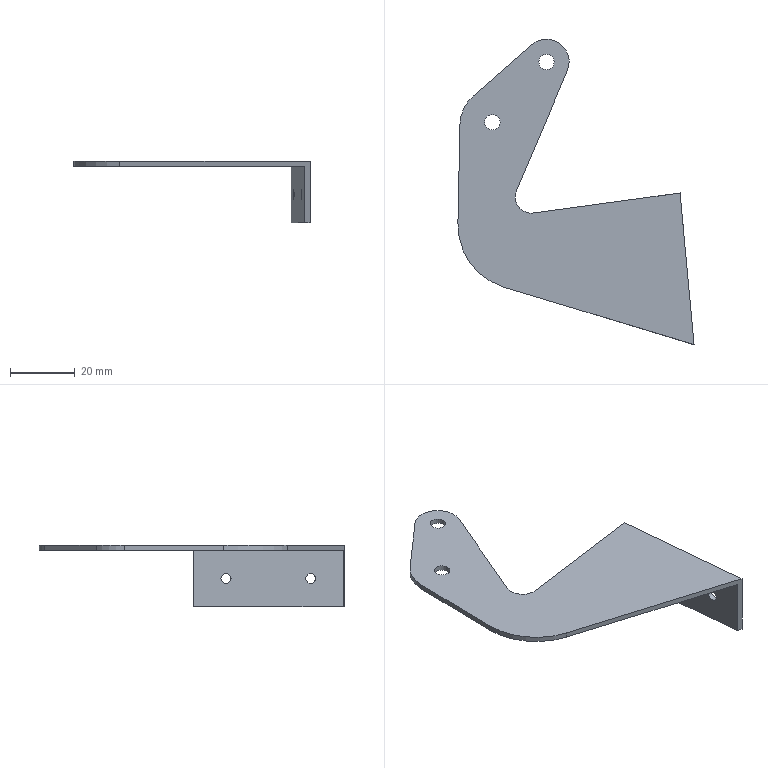Part | NX | features door hinge 2(right) 2 | 1 solid | 18 faces | box 72.896 x 94.255 x 19 mm | volume 6406 mm3 | plane 10 | cylinder 8 | commonest cylinder face diameters 3.175 x2 4.762 x1 4.763 x1 10 x1 14 x1 24 x1
STEP:
#1=CARTESIAN_POINT('',(6.443,-2.735,-1.575));
#2=VERTEX_POINT('',#1);
#3=CARTESIAN_POINT('',(6.443,-2.735,0.));
#4=VERTEX_POINT('',#3);
#5=CARTESIAN_POINT('',(6.443,-2.735,-19.));
#6=DIRECTION('',(0.,0.,1.));
#7=VECTOR('',#6,1000.);
#8=LINE('',#5,#7);
#9=EDGE_CURVE('',#2,#4,#8,.T.);
#10=ORIENTED_EDGE('',*,*,#9,.F.);
#11=CARTESIAN_POINT('',(-4.613,5.265,-1.575));
#12=VERTEX_POINT('',#11);
#13=CARTESIAN_POINT('',(0.,0.,-1.575));
#14=DIRECTION('',(0.,0.,1.));
#15=DIRECTION('',(1.,0.,0.));
#16=AXIS2_PLACEMENT_3D('',#13,#14,#15);
#17=CIRCLE('',#16,7.);
#18=EDGE_CURVE('',#2,#12,#17,.T.);
#19=ORIENTED_EDGE('',*,*,#18,.T.);
#20=CARTESIAN_POINT('',(-4.613,5.265,0.));
#21=VERTEX_POINT('',#20);
#22=CARTESIAN_POINT('',(-4.613,5.265,-19.));
#23=DIRECTION('',(0.,0.,1.));
#24=VECTOR('',#23,1000.);
#25=LINE('',#22,#24);
#26=EDGE_CURVE('',#12,#21,#25,.T.);
#27=ORIENTED_EDGE('',*,*,#26,.T.);
#28=CARTESIAN_POINT('',(0.,0.,0.));
#29=DIRECTION('',(0.,0.,1.));
#30=DIRECTION('',(1.,0.,0.));
#31=AXIS2_PLACEMENT_3D('',#28,#29,#30);
#32=CIRCLE('',#31,7.);
#33=EDGE_CURVE('',#4,#21,#32,.T.);
#34=ORIENTED_EDGE('',*,*,#33,.F.);
#35=EDGE_LOOP('',(#10,#19,#27,#34));
#36=FACE_BOUND('',#35,.T.);
#37=CARTESIAN_POINT('',(0.,0.,-19.));
#38=DIRECTION('',(0.,0.,1.));
#39=DIRECTION('',(1.,0.,0.));
#40=AXIS2_PLACEMENT_3D('',#37,#38,#39);
#41=CYLINDRICAL_SURFACE('',#40,7.);
#42=ADVANCED_FACE('',(#36),#41,.T.);
#43=CARTESIAN_POINT('',(-9.254,-39.713,-1.575));
#44=VERTEX_POINT('',#43);
#45=CARTESIAN_POINT('',(-9.254,-39.713,0.));
#46=VERTEX_POINT('',#45);
#47=CARTESIAN_POINT('',(-9.254,-39.713,-19.));
#48=DIRECTION('',(0.,0.,1.));
#49=VECTOR('',#48,1000.);
#50=LINE('',#47,#49);
#51=EDGE_CURVE('',#44,#46,#50,.T.);
#52=ORIENTED_EDGE('',*,*,#51,.F.);
#53=CARTESIAN_POINT('',(6.443,-2.735,-1.575));
#54=DIRECTION('',(0.3908,0.9205,0.));
#55=VECTOR('',#54,1000.);
#56=LINE('',#53,#55);
#57=EDGE_CURVE('',#44,#2,#56,.T.);
#58=ORIENTED_EDGE('',*,*,#57,.T.);
#59=ORIENTED_EDGE('',*,*,#9,.T.);
#60=CARTESIAN_POINT('',(6.443,-2.735,0.));
#61=DIRECTION('',(0.3908,0.9205,0.));
#62=VECTOR('',#61,1000.);
#63=LINE('',#60,#62);
#64=EDGE_CURVE('',#46,#4,#63,.T.);
#65=ORIENTED_EDGE('',*,*,#64,.F.);
#66=EDGE_LOOP('',(#52,#58,#59,#65));
#67=FACE_BOUND('',#66,.T.);
#68=CARTESIAN_POINT('',(6.443,-2.735,-19.));
#69=DIRECTION('',(0.9205,-0.3908,0.));
#70=DIRECTION('',(0.3908,0.9205,0.));
#71=AXIS2_PLACEMENT_3D('',#68,#69,#70);
#72=PLANE('',#71);
#73=ADVANCED_FACE('',(#67),#72,.T.);
#74=CARTESIAN_POINT('',(-3.976,-46.621,-1.575));
#75=VERTEX_POINT('',#74);
#76=CARTESIAN_POINT('',(-3.976,-46.621,0.));
#77=VERTEX_POINT('',#76);
#78=CARTESIAN_POINT('',(-3.976,-46.621,-19.));
#79=DIRECTION('',(0.,0.,1.));
#80=VECTOR('',#79,1000.);
#81=LINE('',#78,#80);
#82=EDGE_CURVE('',#75,#77,#81,.T.);
#83=ORIENTED_EDGE('',*,*,#82,.F.);
#84=CARTESIAN_POINT('',(-4.652,-41.667,-1.575));
#85=DIRECTION('',(0.,0.,1.));
#86=DIRECTION('',(1.,0.,0.));
#87=AXIS2_PLACEMENT_3D('',#84,#85,#86);
#88=CIRCLE('',#87,5.);
#89=EDGE_CURVE('',#75,#44,#88,.F.);
#90=ORIENTED_EDGE('',*,*,#89,.T.);
#91=ORIENTED_EDGE('',*,*,#51,.T.);
#92=CARTESIAN_POINT('',(-4.652,-41.667,0.));
#93=DIRECTION('',(0.,0.,-1.));
#94=DIRECTION('',(1.,0.,0.));
#95=AXIS2_PLACEMENT_3D('',#92,#93,#94);
#96=CIRCLE('',#95,5.);
#97=EDGE_CURVE('',#77,#46,#96,.T.);
#98=ORIENTED_EDGE('',*,*,#97,.F.);
#99=EDGE_LOOP('',(#83,#90,#91,#98));
#100=FACE_BOUND('',#99,.T.);
#101=CARTESIAN_POINT('',(-4.652,-41.667,-19.));
#102=DIRECTION('',(0.,0.,1.));
#103=DIRECTION('',(1.,0.,0.));
#104=AXIS2_PLACEMENT_3D('',#101,#102,#103);
#105=CYLINDRICAL_SURFACE('',#104,5.);
#106=ADVANCED_FACE('',(#100),#105,.F.);
#107=CARTESIAN_POINT('',(39.663,-40.665,-19.));
#108=VERTEX_POINT('',#107);
#109=CARTESIAN_POINT('',(39.663,-40.665,-1.575));
#110=VERTEX_POINT('',#109);
#111=CARTESIAN_POINT('',(39.663,-40.665,-1.575));
#112=DIRECTION('',(0.,0.,1.));
#113=VECTOR('',#112,1000.);
#114=LINE('',#111,#113);
#115=EDGE_CURVE('',#108,#110,#114,.T.);
#116=ORIENTED_EDGE('',*,*,#115,.T.);
#117=CARTESIAN_POINT('',(6.175,-45.236,-1.575));
#118=DIRECTION('',(-0.9908,-0.1352,0.));
#119=VECTOR('',#118,1000.);
#120=LINE('',#117,#119);
#121=EDGE_CURVE('',#110,#75,#120,.T.);
#122=ORIENTED_EDGE('',*,*,#121,.T.);
#123=ORIENTED_EDGE('',*,*,#82,.T.);
#124=CARTESIAN_POINT('',(41.225,-40.452,0.));
#125=VERTEX_POINT('',#124);
#126=CARTESIAN_POINT('',(-3.976,-46.621,0.));
#127=DIRECTION('',(-0.9908,-0.1352,0.));
#128=VECTOR('',#127,1000.);
#129=LINE('',#126,#128);
#130=EDGE_CURVE('',#125,#77,#129,.T.);
#131=ORIENTED_EDGE('',*,*,#130,.F.);
#132=CARTESIAN_POINT('',(41.225,-40.452,-19.));
#133=VERTEX_POINT('',#132);
#134=CARTESIAN_POINT('',(41.225,-40.452,-1.575));
#135=DIRECTION('',(0.,0.,1.));
#136=VECTOR('',#135,1000.);
#137=LINE('',#134,#136);
#138=EDGE_CURVE('',#133,#125,#137,.T.);
#139=ORIENTED_EDGE('',*,*,#138,.F.);
#140=CARTESIAN_POINT('',(-3.976,-46.621,-19.));
#141=DIRECTION('',(-0.9908,-0.1352,0.));
#142=VECTOR('',#141,1000.);
#143=LINE('',#140,#142);
#144=EDGE_CURVE('',#133,#108,#143,.T.);
#145=ORIENTED_EDGE('',*,*,#144,.T.);
#146=EDGE_LOOP('',(#116,#122,#123,#131,#139,#145));
#147=FACE_BOUND('',#146,.T.);
#148=CARTESIAN_POINT('',(-3.976,-46.621,-19.));
#149=DIRECTION('',(-0.1352,0.9908,0.));
#150=DIRECTION('',(-0.9908,-0.1352,0.));
#151=AXIS2_PLACEMENT_3D('',#148,#149,#150);
#152=PLANE('',#151);
#153=ADVANCED_FACE('',(#147),#152,.T.);
#154=CARTESIAN_POINT('',(-13.139,-69.495,-1.575));
#155=VERTEX_POINT('',#154);
#156=CARTESIAN_POINT('',(-13.139,-69.495,0.));
#157=VERTEX_POINT('',#156);
#158=CARTESIAN_POINT('',(-13.139,-69.495,-19.));
#159=DIRECTION('',(0.,0.,1.));
#160=VECTOR('',#159,1000.);
#161=LINE('',#158,#160);
#162=EDGE_CURVE('',#155,#157,#161,.T.);
#163=ORIENTED_EDGE('',*,*,#162,.F.);
#164=CARTESIAN_POINT('',(43.923,-86.763,-1.575));
#165=VERTEX_POINT('',#164);
#166=CARTESIAN_POINT('',(-20.369,-67.307,-1.575));
#167=DIRECTION('',(0.9571,-0.2897,0.));
#168=VECTOR('',#167,1000.);
#169=LINE('',#166,#168);
#170=EDGE_CURVE('',#155,#165,#169,.T.);
#171=ORIENTED_EDGE('',*,*,#170,.T.);
#172=CARTESIAN_POINT('',(43.923,-86.763,-19.));
#173=VERTEX_POINT('',#172);
#174=CARTESIAN_POINT('',(43.923,-86.763,-19.));
#175=DIRECTION('',(0.,0.,1.));
#176=VECTOR('',#175,1000.);
#177=LINE('',#174,#176);
#178=EDGE_CURVE('',#173,#165,#177,.T.);
#179=ORIENTED_EDGE('',*,*,#178,.F.);
#180=CARTESIAN_POINT('',(45.55,-87.255,-19.));
#181=VERTEX_POINT('',#180);
#182=CARTESIAN_POINT('',(45.551,-87.256,-19.));
#183=DIRECTION('',(0.9571,-0.2897,0.));
#184=VECTOR('',#183,1000.);
#185=LINE('',#182,#184);
#186=EDGE_CURVE('',#173,#181,#185,.T.);
#187=ORIENTED_EDGE('',*,*,#186,.T.);
#188=CARTESIAN_POINT('',(45.55,-87.255,0.));
#189=VERTEX_POINT('',#188);
#190=CARTESIAN_POINT('',(45.55,-87.255,-19.));
#191=DIRECTION('',(0.,0.,1.));
#192=VECTOR('',#191,1000.);
#193=LINE('',#190,#192);
#194=EDGE_CURVE('',#181,#189,#193,.T.);
#195=ORIENTED_EDGE('',*,*,#194,.T.);
#196=CARTESIAN_POINT('',(45.551,-87.256,0.));
#197=DIRECTION('',(0.9571,-0.2897,0.));
#198=VECTOR('',#197,1000.);
#199=LINE('',#196,#198);
#200=EDGE_CURVE('',#157,#189,#199,.T.);
#201=ORIENTED_EDGE('',*,*,#200,.F.);
#202=EDGE_LOOP('',(#163,#171,#179,#187,#195,#201));
#203=FACE_BOUND('',#202,.T.);
#204=CARTESIAN_POINT('',(45.551,-87.256,-19.));
#205=DIRECTION('',(-0.2897,-0.9571,0.));
#206=DIRECTION('',(0.9571,-0.2897,0.));
#207=AXIS2_PLACEMENT_3D('',#204,#205,#206);
#208=PLANE('',#207);
#209=ADVANCED_FACE('',(#203),#208,.T.);
#210=CARTESIAN_POINT('',(-27.342,-49.937,-1.575));
#211=VERTEX_POINT('',#210);
#212=CARTESIAN_POINT('',(-27.342,-49.937,0.));
#213=VERTEX_POINT('',#212);
#214=CARTESIAN_POINT('',(-27.342,-49.937,-19.));
#215=DIRECTION('',(0.,0.,1.));
#216=VECTOR('',#215,1000.);
#217=LINE('',#214,#216);
#218=EDGE_CURVE('',#211,#213,#217,.T.);
#219=ORIENTED_EDGE('',*,*,#218,.F.);
#220=CARTESIAN_POINT('',(-7.346,-50.352,-1.575));
#221=DIRECTION('',(0.,0.,1.));
#222=DIRECTION('',(1.,0.,0.));
#223=AXIS2_PLACEMENT_3D('',#220,#221,#222);
#224=CIRCLE('',#223,20.);
#225=EDGE_CURVE('',#211,#155,#224,.T.);
#226=ORIENTED_EDGE('',*,*,#225,.T.);
#227=ORIENTED_EDGE('',*,*,#162,.T.);
#228=CARTESIAN_POINT('',(-7.346,-50.352,0.));
#229=DIRECTION('',(0.,0.,1.));
#230=DIRECTION('',(1.,0.,0.));
#231=AXIS2_PLACEMENT_3D('',#228,#229,#230);
#232=CIRCLE('',#231,20.);
#233=EDGE_CURVE('',#213,#157,#232,.T.);
#234=ORIENTED_EDGE('',*,*,#233,.F.);
#235=EDGE_LOOP('',(#219,#226,#227,#234));
#236=FACE_BOUND('',#235,.T.);
#237=CARTESIAN_POINT('',(-7.346,-50.352,-19.));
#238=DIRECTION('',(0.,0.,1.));
#239=DIRECTION('',(1.,0.,0.));
#240=AXIS2_PLACEMENT_3D('',#237,#238,#239);
#241=CYLINDRICAL_SURFACE('',#240,20.);
#242=ADVANCED_FACE('',(#236),#241,.T.);
#243=CARTESIAN_POINT('',(-26.706,-19.286,0.));
#244=VERTEX_POINT('',#243);
#245=CARTESIAN_POINT('',(-27.342,-49.937,0.));
#246=DIRECTION('',(-0.02074,-0.9998,0.));
#247=VECTOR('',#246,1000.);
#248=LINE('',#245,#247);
#249=EDGE_CURVE('',#244,#213,#248,.T.);
#250=ORIENTED_EDGE('',*,*,#249,.F.);
#251=CARTESIAN_POINT('',(-26.706,-19.286,-1.575));
#252=VERTEX_POINT('',#251);
#253=CARTESIAN_POINT('',(-26.706,-19.286,-19.));
#254=DIRECTION('',(0.,0.,1.));
#255=VECTOR('',#254,1000.);
#256=LINE('',#253,#255);
#257=EDGE_CURVE('',#244,#252,#256,.F.);
#258=ORIENTED_EDGE('',*,*,#257,.T.);
#259=CARTESIAN_POINT('',(-26.295,0.5454,-1.575));
#260=DIRECTION('',(-0.02074,-0.9998,0.));
#261=VECTOR('',#260,1000.);
#262=LINE('',#259,#261);
#263=EDGE_CURVE('',#252,#211,#262,.T.);
#264=ORIENTED_EDGE('',*,*,#263,.T.);
#265=ORIENTED_EDGE('',*,*,#218,.T.);
#266=EDGE_LOOP('',(#250,#258,#264,#265));
#267=FACE_BOUND('',#266,.T.);
#268=CARTESIAN_POINT('',(-27.342,-49.937,-19.));
#269=DIRECTION('',(-0.9998,0.02074,0.));
#270=DIRECTION('',(-0.02074,-0.9998,0.));
#271=AXIS2_PLACEMENT_3D('',#268,#269,#270);
#272=PLANE('',#271);
#273=ADVANCED_FACE('',(#267),#272,.T.);
#274=CARTESIAN_POINT('',(-22.617,-10.509,-1.575));
#275=VERTEX_POINT('',#274);
#276=CARTESIAN_POINT('',(-4.613,5.265,-1.575));
#277=DIRECTION('',(-0.7521,-0.659,0.));
#278=VECTOR('',#277,1000.);
#279=LINE('',#276,#278);
#280=EDGE_CURVE('',#12,#275,#279,.T.);
#281=ORIENTED_EDGE('',*,*,#280,.T.);
#282=CARTESIAN_POINT('',(-22.617,-10.509,0.));
#283=VERTEX_POINT('',#282);
#284=CARTESIAN_POINT('',(-22.617,-10.509,-19.));
#285=DIRECTION('',(0.,0.,1.));
#286=VECTOR('',#285,1000.);
#287=LINE('',#284,#286);
#288=EDGE_CURVE('',#275,#283,#287,.T.);
#289=ORIENTED_EDGE('',*,*,#288,.T.);
#290=CARTESIAN_POINT('',(-26.597,-13.996,0.));
#291=DIRECTION('',(-0.7521,-0.659,0.));
#292=VECTOR('',#291,1000.);
#293=LINE('',#290,#292);
#294=EDGE_CURVE('',#21,#283,#293,.T.);
#295=ORIENTED_EDGE('',*,*,#294,.F.);
#296=ORIENTED_EDGE('',*,*,#26,.F.);
#297=EDGE_LOOP('',(#281,#289,#295,#296));
#298=FACE_BOUND('',#297,.T.);
#299=CARTESIAN_POINT('',(-26.597,-13.996,-19.));
#300=DIRECTION('',(-0.659,0.7521,0.));
#301=DIRECTION('',(-0.7521,-0.659,0.));
#302=AXIS2_PLACEMENT_3D('',#299,#300,#301);
#303=PLANE('',#302);
#304=ADVANCED_FACE('',(#298),#303,.T.);
#305=CARTESIAN_POINT('',(2.381,0.,0.));
#306=VERTEX_POINT('',#305);
#307=CARTESIAN_POINT('',(0.,0.,0.));
#308=DIRECTION('',(0.,0.,1.));
#309=DIRECTION('',(1.,0.,0.));
#310=AXIS2_PLACEMENT_3D('',#307,#308,#309);
#311=CIRCLE('',#310,2.381);
#312=EDGE_CURVE('',#306,#306,#311,.T.);
#313=ORIENTED_EDGE('',*,*,#312,.T.);
#314=EDGE_LOOP('',(#313));
#315=FACE_BOUND('',#314,.T.);
#316=CARTESIAN_POINT('',(2.381,0.,-1.575));
#317=VERTEX_POINT('',#316);
#318=CARTESIAN_POINT('',(0.,0.,-1.575));
#319=DIRECTION('',(0.,0.,1.));
#320=DIRECTION('',(1.,0.,0.));
#321=AXIS2_PLACEMENT_3D('',#318,#319,#320);
#322=CIRCLE('',#321,2.381);
#323=EDGE_CURVE('',#317,#317,#322,.T.);
#324=ORIENTED_EDGE('',*,*,#323,.F.);
#325=EDGE_LOOP('',(#324));
#326=FACE_BOUND('',#325,.T.);
#327=CARTESIAN_POINT('',(0.,0.,-19.));
#328=DIRECTION('',(0.,0.,1.));
#329=DIRECTION('',(1.,0.,0.));
#330=AXIS2_PLACEMENT_3D('',#327,#328,#329);
#331=CYLINDRICAL_SURFACE('',#330,2.381);
#332=ADVANCED_FACE('',(#315,#326),#331,.F.);
#333=CARTESIAN_POINT('',(-14.309,-18.613,0.));
#334=VERTEX_POINT('',#333);
#335=CARTESIAN_POINT('',(-16.69,-18.613,0.));
#336=DIRECTION('',(0.,0.,1.));
#337=DIRECTION('',(1.,0.,0.));
#338=AXIS2_PLACEMENT_3D('',#335,#336,#337);
#339=CIRCLE('',#338,2.381);
#340=EDGE_CURVE('',#334,#334,#339,.T.);
#341=ORIENTED_EDGE('',*,*,#340,.T.);
#342=EDGE_LOOP('',(#341));
#343=FACE_BOUND('',#342,.T.);
#344=CARTESIAN_POINT('',(-14.309,-18.613,-1.575));
#345=VERTEX_POINT('',#344);
#346=CARTESIAN_POINT('',(-16.69,-18.613,-1.575));
#347=DIRECTION('',(0.,0.,1.));
#348=DIRECTION('',(1.,0.,0.));
#349=AXIS2_PLACEMENT_3D('',#346,#347,#348);
#350=CIRCLE('',#349,2.381);
#351=EDGE_CURVE('',#345,#345,#350,.T.);
#352=ORIENTED_EDGE('',*,*,#351,.F.);
#353=EDGE_LOOP('',(#352));
#354=FACE_BOUND('',#353,.T.);
#355=CARTESIAN_POINT('',(-16.69,-18.613,-19.));
#356=DIRECTION('',(0.,0.,1.));
#357=DIRECTION('',(1.,0.,0.));
#358=AXIS2_PLACEMENT_3D('',#355,#356,#357);
#359=CYLINDRICAL_SURFACE('',#358,2.381);
#360=ADVANCED_FACE('',(#343,#354),#359,.F.);
#361=CARTESIAN_POINT('',(44.425,-75.08,-10.287));
#362=VERTEX_POINT('',#361);
#363=CARTESIAN_POINT('',(44.571,-76.661,-10.287));
#364=DIRECTION('',(0.9958,0.09201,0.));
#365=DIRECTION('',(-0.09201,0.9958,0.));
#366=AXIS2_PLACEMENT_3D('',#363,#364,#365);
#367=CIRCLE('',#366,1.587);
#368=EDGE_CURVE('',#362,#362,#367,.T.);
#369=ORIENTED_EDGE('',*,*,#368,.F.);
#370=EDGE_LOOP('',(#369));
#371=FACE_BOUND('',#370,.T.);
#372=CARTESIAN_POINT('',(42.005,-48.897,-10.287));
#373=VERTEX_POINT('',#372);
#374=CARTESIAN_POINT('',(42.151,-50.477,-10.287));
#375=DIRECTION('',(0.9958,0.09201,0.));
#376=DIRECTION('',(-0.09201,0.9958,0.));
#377=AXIS2_PLACEMENT_3D('',#374,#375,#376);
#378=CIRCLE('',#377,1.587);
#379=EDGE_CURVE('',#373,#373,#378,.T.);
#380=ORIENTED_EDGE('',*,*,#379,.F.);
#381=EDGE_LOOP('',(#380));
#382=FACE_BOUND('',#381,.T.);
#383=CARTESIAN_POINT('',(37.17,3.435,0.));
#384=DIRECTION('',(-0.09201,0.9958,0.));
#385=VECTOR('',#384,1000.);
#386=LINE('',#383,#385);
#387=EDGE_CURVE('',#189,#125,#386,.T.);
#388=ORIENTED_EDGE('',*,*,#387,.F.);
#389=ORIENTED_EDGE('',*,*,#194,.F.);
#390=CARTESIAN_POINT('',(37.17,3.435,-19.));
#391=DIRECTION('',(-0.09201,0.9958,0.));
#392=VECTOR('',#391,1000.);
#393=LINE('',#390,#392);
#394=EDGE_CURVE('',#181,#133,#393,.T.);
#395=ORIENTED_EDGE('',*,*,#394,.T.);
#396=ORIENTED_EDGE('',*,*,#138,.T.);
#397=EDGE_LOOP('',(#388,#389,#395,#396));
#398=FACE_BOUND('',#397,.T.);
#399=CARTESIAN_POINT('',(41.231,-40.52,-1.575));
#400=DIRECTION('',(0.9958,0.09201,0.));
#401=DIRECTION('',(-0.09201,0.9958,0.));
#402=AXIS2_PLACEMENT_3D('',#399,#400,#401);
#403=PLANE('',#402);
#404=ADVANCED_FACE('',(#371,#382,#398),#403,.T.);
#405=ORIENTED_EDGE('',*,*,#186,.F.);
#406=CARTESIAN_POINT('',(35.601,3.29,-19.));
#407=DIRECTION('',(-0.09201,0.9958,0.));
#408=VECTOR('',#407,1000.);
#409=LINE('',#406,#408);
#410=EDGE_CURVE('',#173,#108,#409,.T.);
#411=ORIENTED_EDGE('',*,*,#410,.T.);
#412=ORIENTED_EDGE('',*,*,#144,.F.);
#413=ORIENTED_EDGE('',*,*,#394,.F.);
#414=EDGE_LOOP('',(#405,#411,#412,#413));
#415=FACE_BOUND('',#414,.T.);
#416=CARTESIAN_POINT('',(0.,0.,-19.));
#417=DIRECTION('',(0.,0.,1.));
#418=DIRECTION('',(1.,0.,0.));
#419=AXIS2_PLACEMENT_3D('',#416,#417,#418);
#420=PLANE('',#419);
#421=ADVANCED_FACE('',(#415),#420,.F.);
#422=ORIENTED_EDGE('',*,*,#340,.F.);
#423=EDGE_LOOP('',(#422));
#424=FACE_BOUND('',#423,.T.);
#425=ORIENTED_EDGE('',*,*,#312,.F.);
#426=EDGE_LOOP('',(#425));
#427=FACE_BOUND('',#426,.T.);
#428=ORIENTED_EDGE('',*,*,#294,.T.);
#429=CARTESIAN_POINT('',(-14.709,-19.535,0.));
#430=DIRECTION('',(0.,0.,1.));
#431=DIRECTION('',(1.,0.,0.));
#432=AXIS2_PLACEMENT_3D('',#429,#430,#431);
#433=CIRCLE('',#432,12.);
#434=EDGE_CURVE('',#283,#244,#433,.T.);
#435=ORIENTED_EDGE('',*,*,#434,.T.);
#436=ORIENTED_EDGE('',*,*,#249,.T.);
#437=ORIENTED_EDGE('',*,*,#233,.T.);
#438=ORIENTED_EDGE('',*,*,#200,.T.);
#439=ORIENTED_EDGE('',*,*,#387,.T.);
#440=ORIENTED_EDGE('',*,*,#130,.T.);
#441=ORIENTED_EDGE('',*,*,#97,.T.);
#442=ORIENTED_EDGE('',*,*,#64,.T.);
#443=ORIENTED_EDGE('',*,*,#33,.T.);
#444=EDGE_LOOP('',(#428,#435,#436,#437,#438,#439,#440,#441,#442,#443));
#445=FACE_BOUND('',#444,.T.);
#446=CARTESIAN_POINT('',(0.,0.,0.));
#447=DIRECTION('',(0.,0.,1.));
#448=DIRECTION('',(1.,0.,0.));
#449=AXIS2_PLACEMENT_3D('',#446,#447,#448);
#450=PLANE('',#449);
#451=ADVANCED_FACE('',(#424,#427,#445),#450,.T.);
#452=CARTESIAN_POINT('',(42.856,-75.225,-10.287));
#453=VERTEX_POINT('',#452);
#454=CARTESIAN_POINT('',(43.003,-76.805,-10.287));
#455=DIRECTION('',(0.9958,0.09201,0.));
#456=DIRECTION('',(-0.09201,0.9958,0.));
#457=AXIS2_PLACEMENT_3D('',#454,#455,#456);
#458=CIRCLE('',#457,1.587);
#459=EDGE_CURVE('',#453,#453,#458,.T.);
#460=ORIENTED_EDGE('',*,*,#459,.T.);
#461=EDGE_LOOP('',(#460));
#462=FACE_BOUND('',#461,.T.);
#463=CARTESIAN_POINT('',(40.437,-49.042,-10.287));
#464=VERTEX_POINT('',#463);
#465=CARTESIAN_POINT('',(40.583,-50.622,-10.287));
#466=DIRECTION('',(0.9958,0.09201,0.));
#467=DIRECTION('',(-0.09201,0.9958,0.));
#468=AXIS2_PLACEMENT_3D('',#465,#466,#467);
#469=CIRCLE('',#468,1.587);
#470=EDGE_CURVE('',#464,#464,#469,.T.);
#471=ORIENTED_EDGE('',*,*,#470,.T.);
#472=EDGE_LOOP('',(#471));
#473=FACE_BOUND('',#472,.T.);
#474=ORIENTED_EDGE('',*,*,#178,.T.);
#475=CARTESIAN_POINT('',(35.601,3.29,-1.575));
#476=DIRECTION('',(-0.09201,0.9958,0.));
#477=VECTOR('',#476,1000.);
#478=LINE('',#475,#477);
#479=EDGE_CURVE('',#165,#110,#478,.T.);
#480=ORIENTED_EDGE('',*,*,#479,.T.);
#481=ORIENTED_EDGE('',*,*,#115,.F.);
#482=ORIENTED_EDGE('',*,*,#410,.F.);
#483=EDGE_LOOP('',(#474,#480,#481,#482));
#484=FACE_BOUND('',#483,.T.);
#485=CARTESIAN_POINT('',(39.663,-40.665,-1.575));
#486=DIRECTION('',(0.9958,0.09201,0.));
#487=DIRECTION('',(-0.09201,0.9958,0.));
#488=AXIS2_PLACEMENT_3D('',#485,#486,#487);
#489=PLANE('',#488);
#490=ADVANCED_FACE('',(#462,#473,#484),#489,.F.);
#491=ORIENTED_EDGE('',*,*,#351,.T.);
#492=EDGE_LOOP('',(#491));
#493=FACE_BOUND('',#492,.T.);
#494=ORIENTED_EDGE('',*,*,#323,.T.);
#495=EDGE_LOOP('',(#494));
#496=FACE_BOUND('',#495,.T.);
#497=ORIENTED_EDGE('',*,*,#121,.F.);
#498=ORIENTED_EDGE('',*,*,#479,.F.);
#499=ORIENTED_EDGE('',*,*,#170,.F.);
#500=ORIENTED_EDGE('',*,*,#225,.F.);
#501=ORIENTED_EDGE('',*,*,#263,.F.);
#502=CARTESIAN_POINT('',(-14.709,-19.535,-1.575));
#503=DIRECTION('',(0.,0.,1.));
#504=DIRECTION('',(1.,0.,0.));
#505=AXIS2_PLACEMENT_3D('',#502,#503,#504);
#506=CIRCLE('',#505,12.);
#507=EDGE_CURVE('',#252,#275,#506,.F.);
#508=ORIENTED_EDGE('',*,*,#507,.T.);
#509=ORIENTED_EDGE('',*,*,#280,.F.);
#510=ORIENTED_EDGE('',*,*,#18,.F.);
#511=ORIENTED_EDGE('',*,*,#57,.F.);
#512=ORIENTED_EDGE('',*,*,#89,.F.);
#513=EDGE_LOOP('',(#497,#498,#499,#500,#501,#508,#509,#510,#511,#512));
#514=FACE_BOUND('',#513,.T.);
#515=CARTESIAN_POINT('',(0.,0.,-1.575));
#516=DIRECTION('',(0.,0.,1.));
#517=DIRECTION('',(1.,0.,0.));
#518=AXIS2_PLACEMENT_3D('',#515,#516,#517);
#519=PLANE('',#518);
#520=ADVANCED_FACE('',(#493,#496,#514),#519,.F.);
#521=ORIENTED_EDGE('',*,*,#507,.F.);
#522=ORIENTED_EDGE('',*,*,#257,.F.);
#523=ORIENTED_EDGE('',*,*,#434,.F.);
#524=ORIENTED_EDGE('',*,*,#288,.F.);
#525=EDGE_LOOP('',(#521,#522,#523,#524));
#526=FACE_BOUND('',#525,.T.);
#527=CARTESIAN_POINT('',(-14.709,-19.535,-19.));
#528=DIRECTION('',(0.,0.,1.));
#529=DIRECTION('',(1.,0.,0.));
#530=AXIS2_PLACEMENT_3D('',#527,#528,#529);
#531=CYLINDRICAL_SURFACE('',#530,12.);
#532=ADVANCED_FACE('',(#526),#531,.T.);
#533=ORIENTED_EDGE('',*,*,#379,.T.);
#534=EDGE_LOOP('',(#533));
#535=FACE_BOUND('',#534,.T.);
#536=ORIENTED_EDGE('',*,*,#470,.F.);
#537=EDGE_LOOP('',(#536));
#538=FACE_BOUND('',#537,.T.);
#539=CARTESIAN_POINT('',(40.583,-50.622,-10.287));
#540=DIRECTION('',(0.9958,0.09201,0.));
#541=DIRECTION('',(-0.09201,0.9958,0.));
#542=AXIS2_PLACEMENT_3D('',#539,#540,#541);
#543=CYLINDRICAL_SURFACE('',#542,1.587);
#544=ADVANCED_FACE('',(#535,#538),#543,.F.);
#545=ORIENTED_EDGE('',*,*,#368,.T.);
#546=EDGE_LOOP('',(#545));
#547=FACE_BOUND('',#546,.T.);
#548=ORIENTED_EDGE('',*,*,#459,.F.);
#549=EDGE_LOOP('',(#548));
#550=FACE_BOUND('',#549,.T.);
#551=CARTESIAN_POINT('',(43.003,-76.805,-10.287));
#552=DIRECTION('',(0.9958,0.09201,0.));
#553=DIRECTION('',(-0.09201,0.9958,0.));
#554=AXIS2_PLACEMENT_3D('',#551,#552,#553);
#555=CYLINDRICAL_SURFACE('',#554,1.587);
#556=ADVANCED_FACE('',(#547,#550),#555,.F.);
#557=CLOSED_SHELL('',(#42,#73,#106,#153,#209,#242,#273,#304,#332,#360,#404,#421,#451,#490,#520,#532,#544,#556));
#558=MANIFOLD_SOLID_BREP('',#557);
#559=(LENGTH_UNIT()NAMED_UNIT(*)SI_UNIT(.MILLI.,.METRE.));
#560=UNCERTAINTY_MEASURE_WITH_UNIT(LENGTH_MEASURE(0.00001),#559,'','');
#561=(NAMED_UNIT(*)PLANE_ANGLE_UNIT()SI_UNIT($,.RADIAN.));
#562=(NAMED_UNIT(*)SI_UNIT($,.STERADIAN.)SOLID_ANGLE_UNIT());
#563=(GEOMETRIC_REPRESENTATION_CONTEXT(3)GLOBAL_UNCERTAINTY_ASSIGNED_CONTEXT((#560))GLOBAL_UNIT_ASSIGNED_CONTEXT((#559,#561,#562))REPRESENTATION_CONTEXT('',''));
#564=ADVANCED_BREP_SHAPE_REPRESENTATION('',(#558),#563);